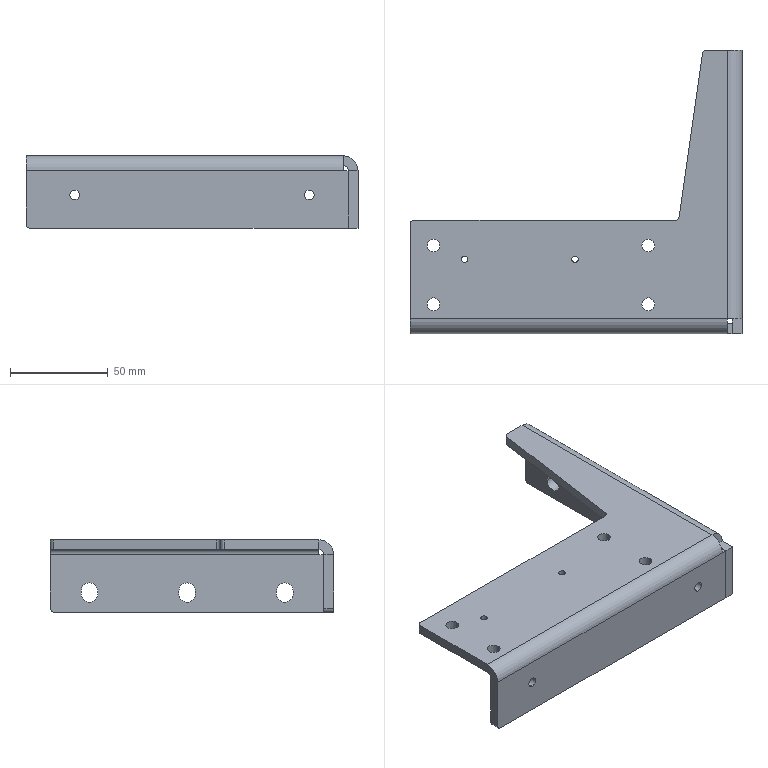Part | STEP file | 1 solid | 62 faces | box 170 x 145 x 37 mm | volume 104662 mm3 | cylinder 34 | plane 28 | commonest cylinder face diameters 8.5 x9 6.5 x8 5 x6 4 x5 3.3 x4 15 x2